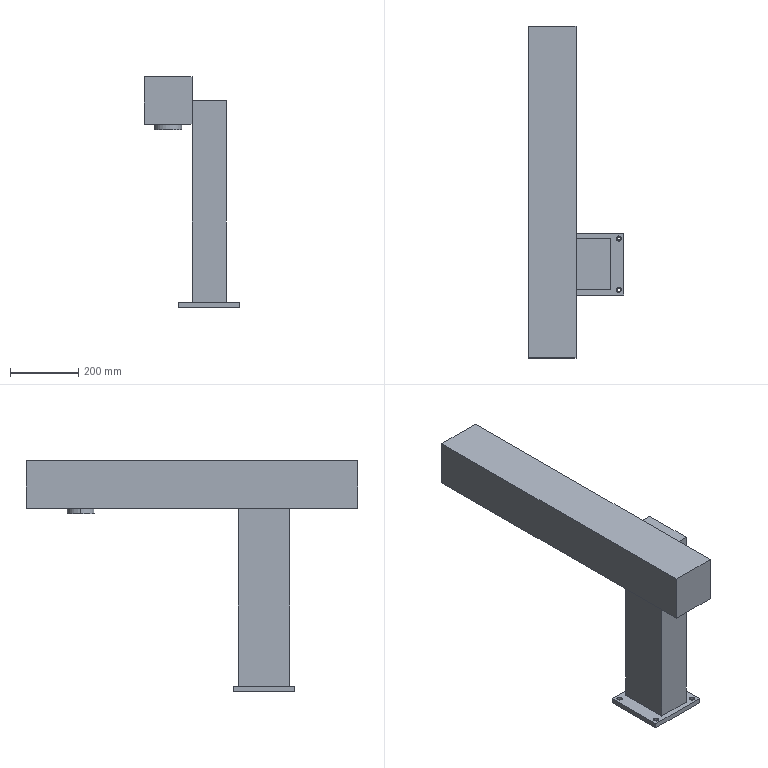Part | STEP file | Ultrasonic welding | 3 solids | 41 faces | box 280 x 970 x 675 mm | volume 28415691 mm3 | plane 23 | cylinder 18 | commonest cylinder face diameters 9 x8 15 x8 80 x2